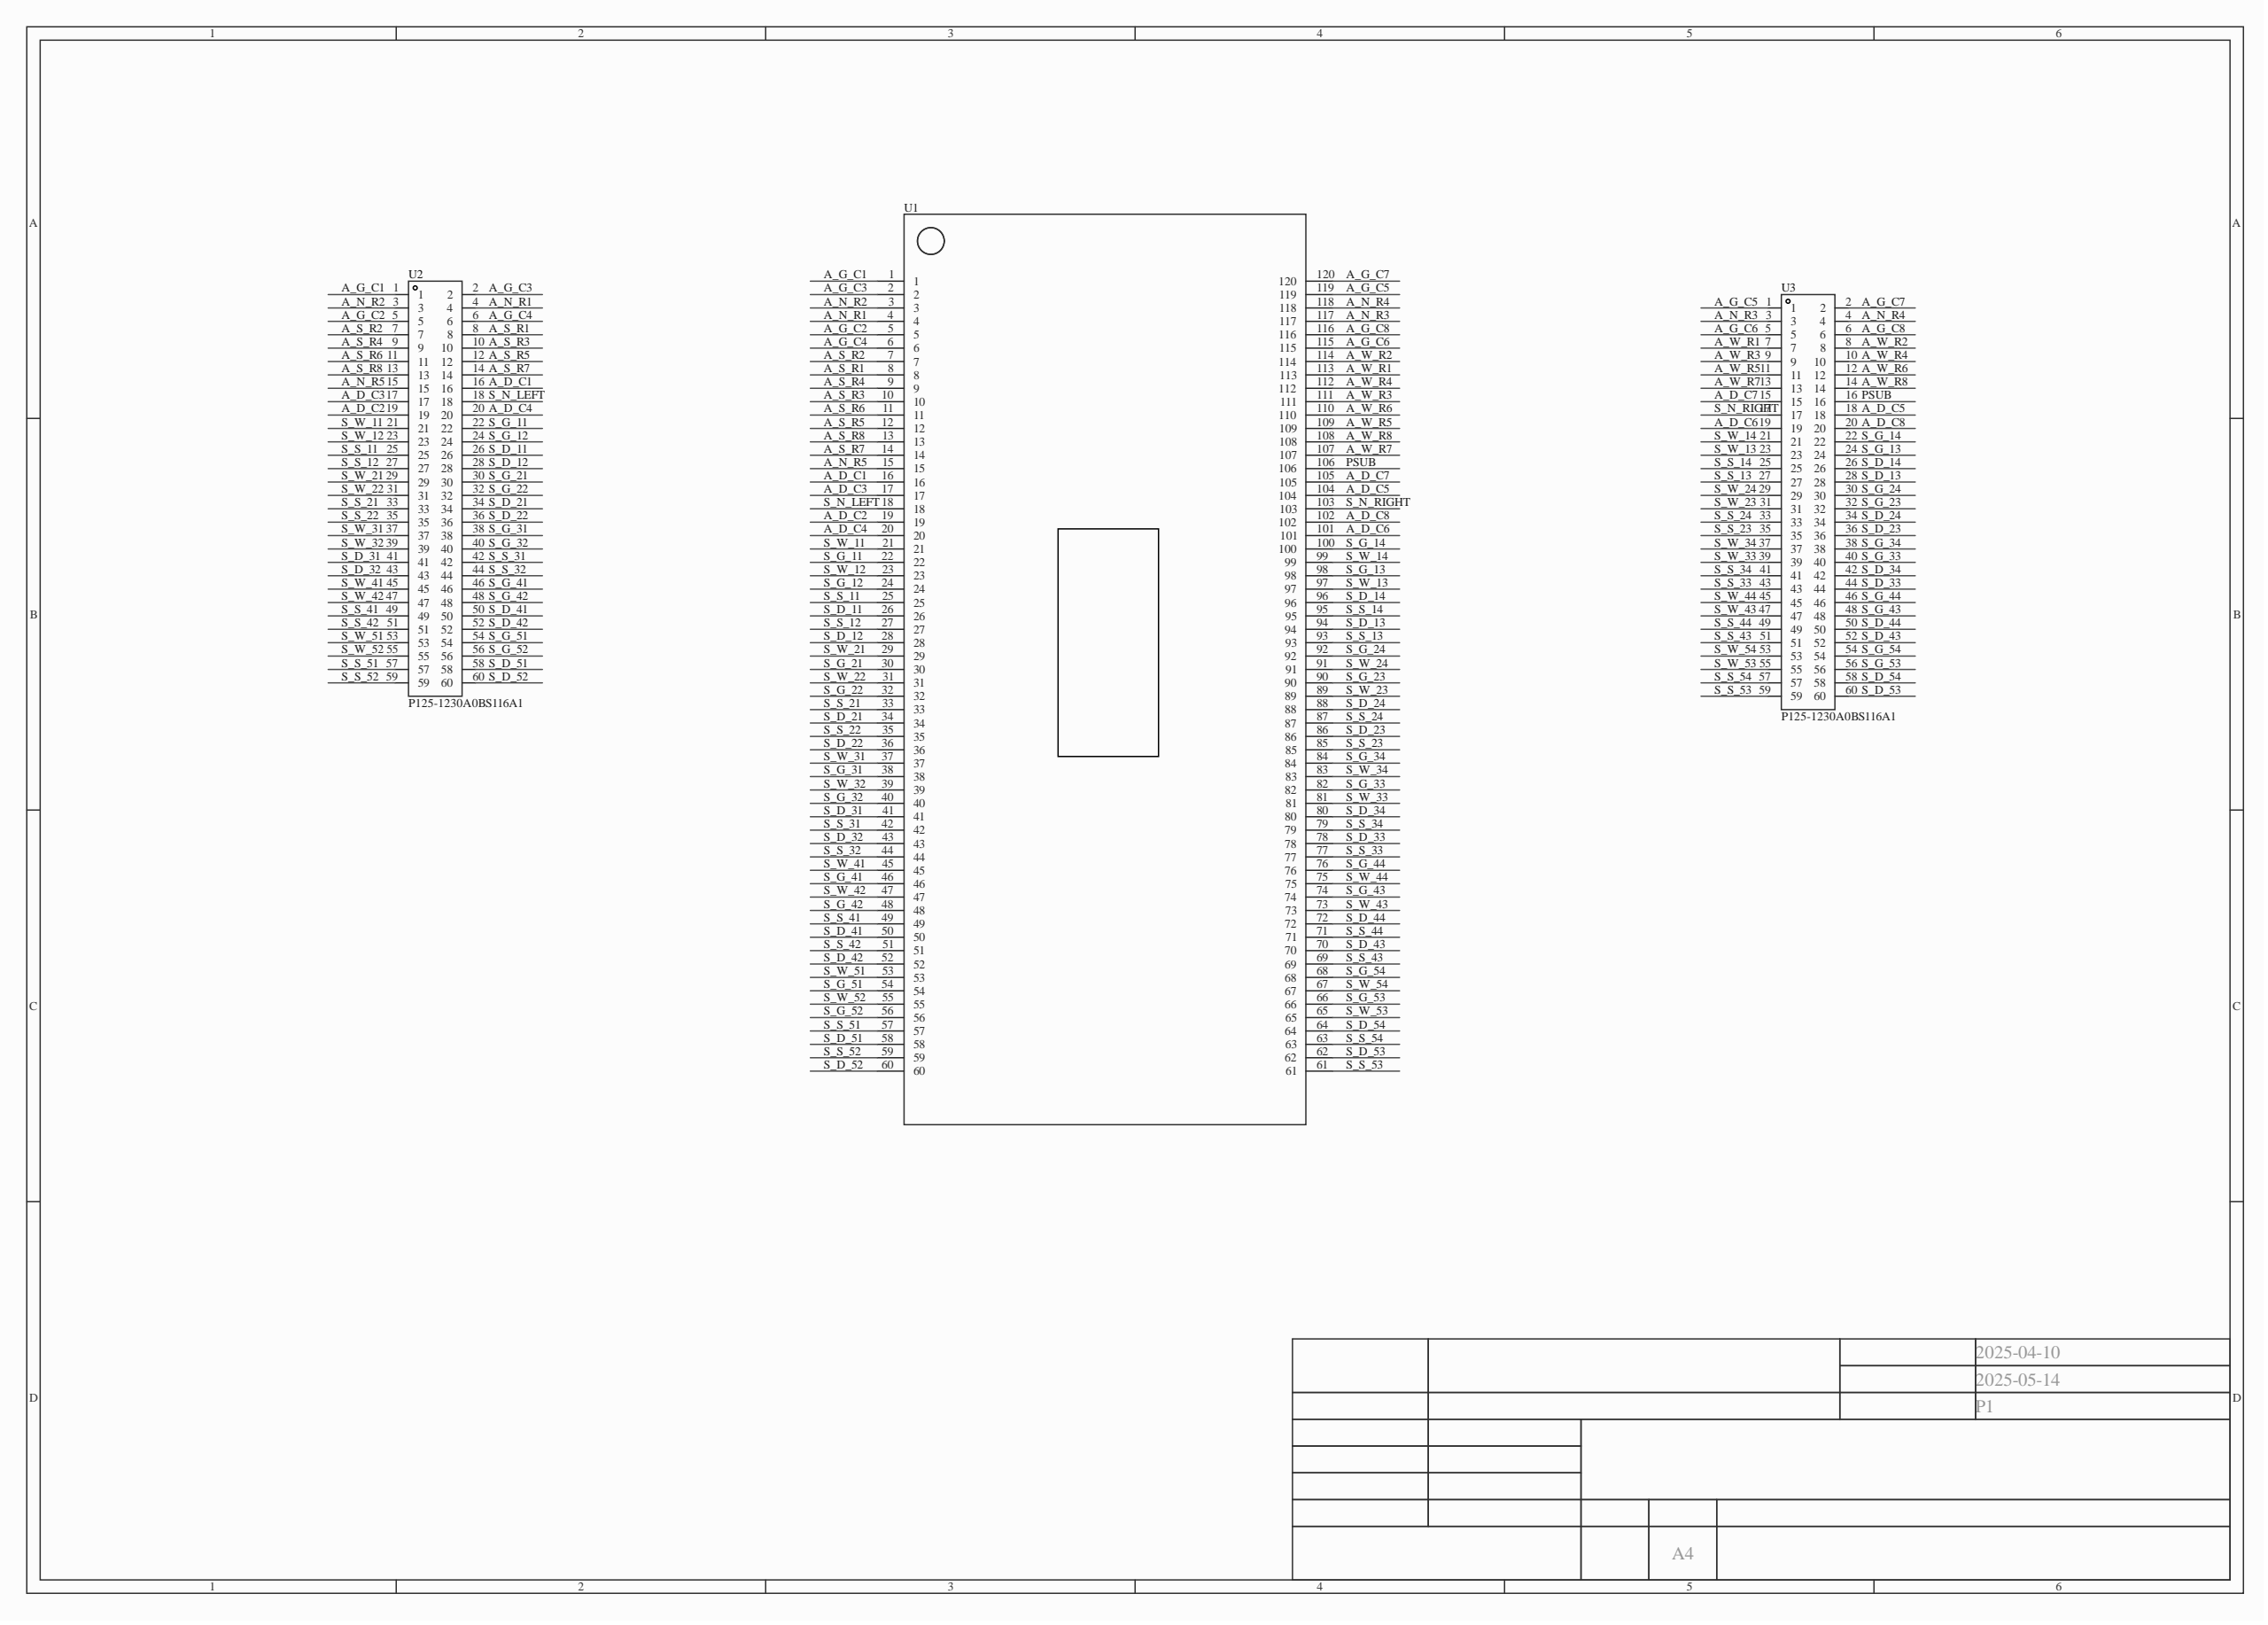Circuit board | Altium Designer | 3 parts | 120 nets
Bill of materials:
Comment,Description,Designator,Footprint,LibRef,Quantity
"","","U1","XP","Chip3Array","1"
"P125-1230A0BS116A1","","U2, U3","HDR-TH_60P-P2.54-V-M-R2-C30-S2.54-1","P125-1230A0BS116A1","2"
Netlist (Protel format):
[
U1
XP




]
[
U2
HDR-TH_60P-P2.54-V-M-R2-C30-S2.54-1
P125-1230A0BS116A1



]
[
U3
HDR-TH_60P-P2.54-V-M-R2-C30-S2.54-1
P125-1230A0BS116A1



]
(
S_W_54
U1-67
U3-53
)
(
S_W_53
U1-65
U3-55
)
(
S_W_52
U1-55
U2-55
)
(
S_W_51
U1-53
U2-53
)
(
S_W_44
U1-75
U3-45
)
(
S_W_43
U1-73
U3-47
)
(
S_W_42
U1-47
U2-47
)
(
S_W_41
U1-45
U2-45
)
(
S_W_34
U1-83
U3-37
)
(
S_W_33
U1-81
U3-39
)
(
S_W_32
U1-39
U2-39
)
(
S_W_31
U1-37
U2-37
)
(
S_W_24
U1-91
U3-29
)
(
S_W_23
U1-89
U3-31
)
(
S_W_22
U1-31
U2-31
)
(
S_W_21
U1-29
U2-29
)
(
S_W_14
U1-99
U3-21
)
(
S_W_13
U1-97
U3-23
)
(
S_W_12
U1-23
U2-23
)
(
S_W_11
U1-21
U2-21
)
(
S_S_54
U1-63
U3-57
)
(
S_S_53
U1-61
U3-59
)
(
S_S_52
U1-59
U2-59
)
(
S_S_51
U1-57
U2-57
)
(
S_S_44
U1-71
U3-49
)
(
S_S_43
U1-69
U3-51
)
(
S_S_42
U1-51
U2-51
)
(
S_S_41
U1-49
U2-49
)
(
S_S_34
U1-79
U3-41
)
(
S_S_33
U1-77
U3-43
)
(
S_S_32
U1-44
U2-44
)
(
S_S_31
U1-42
U2-42
)
(
S_S_24
U1-87
U3-33
)
(
S_S_23
U1-85
U3-35
)
(
S_S_22
U1-35
U2-35
)
(
S_S_21
U1-33
U2-33
)
(
S_S_14
U1-95
U3-25
)
(
S_S_13
U1-93
U3-27
)
(
S_S_12
U1-27
U2-27
)
(
S_S_11
U1-25
U2-25
)
(
S_N_RIGHT
U1-103
U3-17
)
(
S_N_LEFT
U1-18
U2-18
)
(
S_G_54
U1-68
U3-54
)
(
S_G_53
U1-66
U3-56
)
(
S_G_52
U1-56
U2-56
)
(
S_G_51
U1-54
U2-54
)
(
S_G_44
U1-76
U3-46
)
(
S_G_43
U1-74
U3-48
)
(
S_G_42
U1-48
U2-48
)
(
S_G_41
U1-46
U2-46
)
(
S_G_34
U1-84
U3-38
)
(
S_G_33
U1-82
U3-40
)
(
S_G_32
U1-40
U2-40
)
(
S_G_31
U1-38
U2-38
)
(
S_G_24
U1-92
U3-30
)
(
S_G_23
U1-90
U3-32
)
(
S_G_22
U1-32
U2-32
)
(
S_G_21
U1-30
U2-30
)
(
S_G_14
U1-100
U3-22
)
(
S_G_13
U1-98
U3-24
)
(
S_G_12
U1-24
U2-24
)
(
S_G_11
U1-22
U2-22
)
(
S_D_54
U1-64
U3-58
)
(
S_D_53
U1-62
U3-60
)
(
S_D_52
U1-60
U2-60
)
(
S_D_51
U1-58
U2-58
)
(
S_D_44
U1-72
U3-50
)
(
S_D_43
U1-70
U3-52
)
(
S_D_42
U1-52
U2-52
)
(
S_D_41
U1-50
U2-50
)
(
S_D_34
U1-80
U3-42
)
(
S_D_33
U1-78
U3-44
)
(
S_D_32
U1-43
U2-43
)
(
S_D_31
U1-41
U2-41
)
(
S_D_24
U1-88
U3-34
)
(
S_D_23
U1-86
U3-36
)
(
S_D_22
U1-36
U2-36
)
(
S_D_21
U1-34
U2-34
)
(
S_D_14
U1-96
U3-26
)
(
S_D_13
U1-94
U3-28
)
(
S_D_12
U1-28
U2-28
)
(
S_D_11
U1-26
U2-26
)
(
PSUB
U1-106
U3-16
)
(
A_W_R8
U1-108
U3-14
)
(
A_W_R7
U1-107
U3-13
)
(
A_W_R6
U1-110
U3-12
)
(
A_W_R5
U1-109
U3-11
)
(
A_W_R4
U1-112
U3-10
)
(
A_W_R3
U1-111
U3-9
)
(
A_W_R2
U1-114
U3-8
)
(
A_W_R1
U1-113
U3-7
)
(
A_S_R8
U1-13
U2-13
)
(
A_S_R7
U1-14
U2-14
)
(
A_S_R6
U1-11
U2-11
)
(
A_S_R5
U1-12
U2-12
)
(
A_S_R4
U1-9
U2-9
)
(
A_S_R3
U1-10
U2-10
)
(
A_S_R2
U1-7
U2-7
)
(
A_S_R1
U1-8
U2-8
)
(
A_N_R5
U1-15
U2-15
)
(
A_N_R4
U1-118
U3-4
)
(
A_N_R3
U1-117
U3-3
)
(
A_N_R2
U1-3
U2-3
)
(
A_N_R1
U1-4
U2-4
)
(
A_G_C8
U1-116
U3-6
)
(
A_G_C7
U1-120
U3-2
)
(
A_G_C6
U1-115
U3-5
)
(
A_G_C5
U1-119
U3-1
)
(
A_G_C4
U1-6
U2-6
)
(
A_G_C3
U1-2
U2-2
)
(
A_G_C2
U1-5
U2-5
)
(
A_G_C1
U1-1
U2-1
)
(
A_D_C8
U1-102
U3-20
)
(
A_D_C7
U1-105
U3-15
)
(
A_D_C6
U1-101
U3-19
)
(
A_D_C5
U1-104
U3-18
)
(
A_D_C4
U1-20
U2-20
)
(
A_D_C3
U1-17
U2-17
)
(
A_D_C2
U1-19
U2-19
)
(
A_D_C1
U1-16
U2-16
)